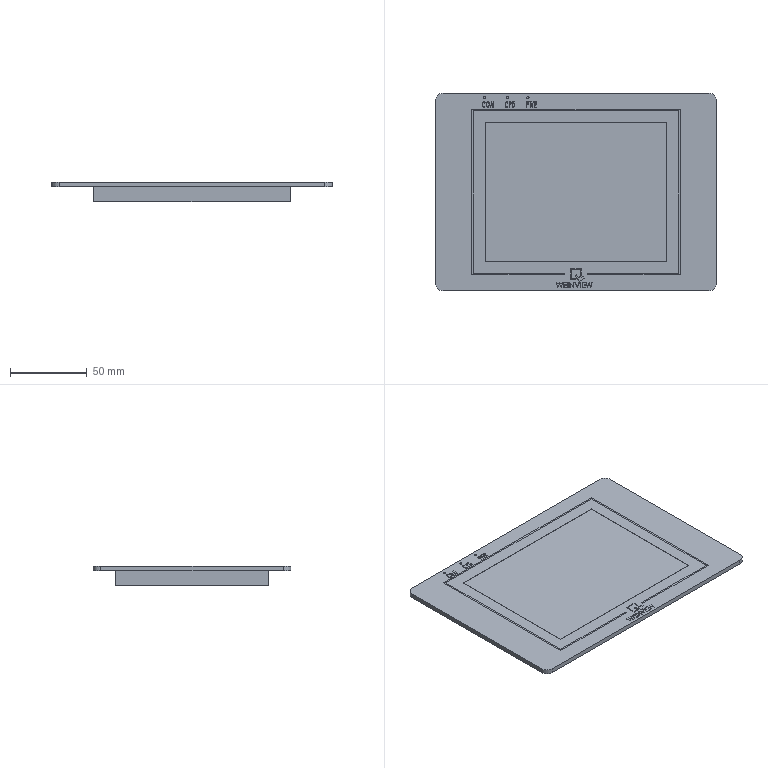Part | SolidWorks | features BaseBody 26 | 26 solids | 570 faces | box 183 x 129 x 13 mm | volume 196633 mm3 | plane 446 | spline 108 | cylinder 16 | commonest cylinder face diameters 1.5 x12 10 x4